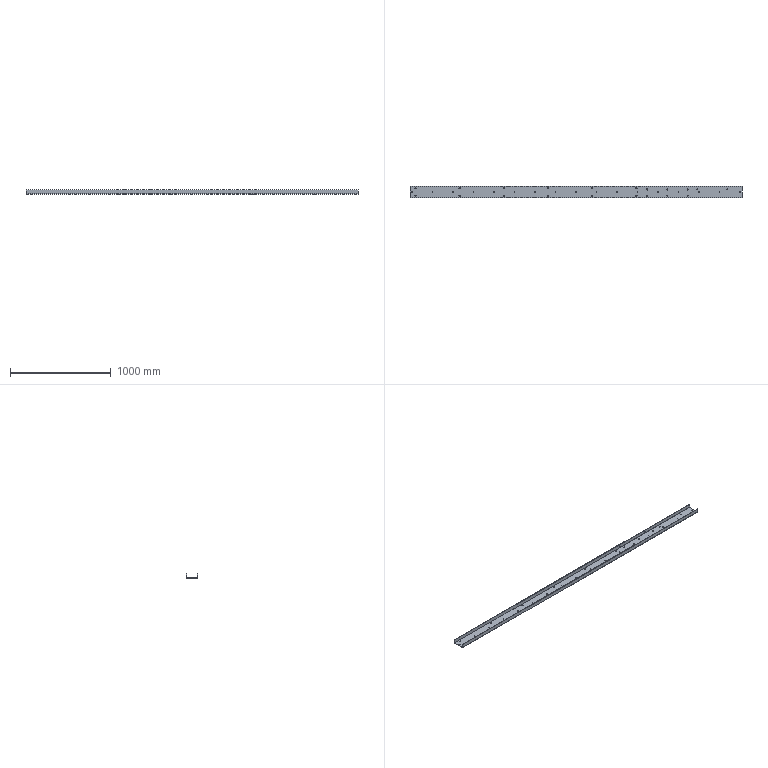Part | STEP file | Mirror SX-001-02 | 1 solid | 136 faces | box 3291 x 117 x 40 mm | volume 3023077 mm3 | cylinder 94 | plane 42 | commonest cylinder face diameters 10 x40 8 x38 10.5 x12 0.4 x2 10.4 x2